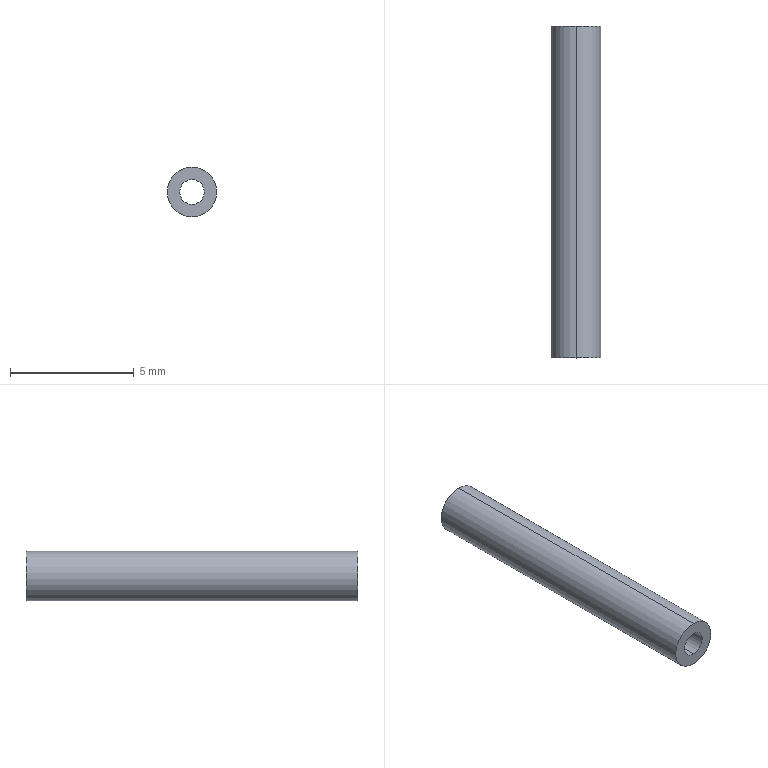Part | SolidWorks | features Extrusion 1 | 1 solid | 6 faces | box 2 x 13.4 x 2 mm | volume 31.573 mm3 | cylinder 4 | plane 2 | commonest cylinder face diameters 1 x2 2 x2
STEP:
#1=CARTESIAN_POINT('',(0.,13.4,-0.5));
#2=VERTEX_POINT('',#1);
#3=CARTESIAN_POINT('',(0.,13.4,0.5));
#4=VERTEX_POINT('',#3);
#5=CARTESIAN_POINT('',(0.,13.4,0.));
#6=DIRECTION('',(0.,1.,0.));
#7=DIRECTION('',(0.,0.,1.));
#8=AXIS2_PLACEMENT_3D('',#5,#6,#7);
#9=CIRCLE('',#8,0.5);
#10=EDGE_CURVE('',#2,#4,#9,.T.);
#11=ORIENTED_EDGE('',*,*,#10,.T.);
#12=CARTESIAN_POINT('',(0.,0.,0.5));
#13=VERTEX_POINT('',#12);
#14=CARTESIAN_POINT('',(0.,13.4,0.5));
#15=DIRECTION('',(0.,-1.,0.));
#16=VECTOR('',#15,1000.);
#17=LINE('',#14,#16);
#18=EDGE_CURVE('',#4,#13,#17,.T.);
#19=ORIENTED_EDGE('',*,*,#18,.T.);
#20=CARTESIAN_POINT('',(0.,0.,-0.5));
#21=VERTEX_POINT('',#20);
#22=CARTESIAN_POINT('',(0.,0.,0.));
#23=DIRECTION('',(0.,1.,0.));
#24=DIRECTION('',(0.,0.,1.));
#25=AXIS2_PLACEMENT_3D('',#22,#23,#24);
#26=CIRCLE('',#25,0.5);
#27=EDGE_CURVE('',#21,#13,#26,.T.);
#28=ORIENTED_EDGE('',*,*,#27,.F.);
#29=CARTESIAN_POINT('',(0.,13.4,-0.5));
#30=DIRECTION('',(0.,-1.,0.));
#31=VECTOR('',#30,1000.);
#32=LINE('',#29,#31);
#33=EDGE_CURVE('',#2,#21,#32,.T.);
#34=ORIENTED_EDGE('',*,*,#33,.F.);
#35=EDGE_LOOP('',(#11,#19,#28,#34));
#36=FACE_OUTER_BOUND('',#35,.T.);
#37=CARTESIAN_POINT('',(0.,13.4,0.));
#38=DIRECTION('',(0.,-1.,0.));
#39=DIRECTION('',(0.,0.,-1.));
#40=AXIS2_PLACEMENT_3D('',#37,#38,#39);
#41=CYLINDRICAL_SURFACE('',#40,0.5);
#42=ADVANCED_FACE('',(#36),#41,.F.);
#43=CARTESIAN_POINT('',(0.,13.4,1.));
#44=VERTEX_POINT('',#43);
#45=CARTESIAN_POINT('',(0.,13.4,-1.));
#46=VERTEX_POINT('',#45);
#47=CARTESIAN_POINT('',(0.,13.4,0.));
#48=DIRECTION('',(0.,1.,0.));
#49=DIRECTION('',(0.,0.,1.));
#50=AXIS2_PLACEMENT_3D('',#47,#48,#49);
#51=CIRCLE('',#50,1.);
#52=EDGE_CURVE('',#44,#46,#51,.T.);
#53=ORIENTED_EDGE('',*,*,#52,.F.);
#54=CARTESIAN_POINT('',(0.,0.,1.));
#55=VERTEX_POINT('',#54);
#56=CARTESIAN_POINT('',(0.,13.4,1.));
#57=DIRECTION('',(0.,-1.,0.));
#58=VECTOR('',#57,1000.);
#59=LINE('',#56,#58);
#60=EDGE_CURVE('',#44,#55,#59,.T.);
#61=ORIENTED_EDGE('',*,*,#60,.T.);
#62=CARTESIAN_POINT('',(0.,0.,-1.));
#63=VERTEX_POINT('',#62);
#64=CARTESIAN_POINT('',(0.,0.,0.));
#65=DIRECTION('',(0.,1.,0.));
#66=DIRECTION('',(0.,0.,1.));
#67=AXIS2_PLACEMENT_3D('',#64,#65,#66);
#68=CIRCLE('',#67,1.);
#69=EDGE_CURVE('',#55,#63,#68,.T.);
#70=ORIENTED_EDGE('',*,*,#69,.T.);
#71=CARTESIAN_POINT('',(0.,13.4,-1.));
#72=DIRECTION('',(0.,-1.,0.));
#73=VECTOR('',#72,1000.);
#74=LINE('',#71,#73);
#75=EDGE_CURVE('',#46,#63,#74,.T.);
#76=ORIENTED_EDGE('',*,*,#75,.F.);
#77=EDGE_LOOP('',(#53,#61,#70,#76));
#78=FACE_OUTER_BOUND('',#77,.T.);
#79=CARTESIAN_POINT('',(0.,13.4,0.));
#80=DIRECTION('',(0.,-1.,0.));
#81=DIRECTION('',(0.,0.,-1.));
#82=AXIS2_PLACEMENT_3D('',#79,#80,#81);
#83=CYLINDRICAL_SURFACE('',#82,1.);
#84=ADVANCED_FACE('',(#78),#83,.T.);
#85=CARTESIAN_POINT('',(0.,13.4,0.));
#86=DIRECTION('',(0.,1.,0.));
#87=DIRECTION('',(0.,0.,1.));
#88=AXIS2_PLACEMENT_3D('',#85,#86,#87);
#89=CIRCLE('',#88,1.);
#90=EDGE_CURVE('',#46,#44,#89,.T.);
#91=ORIENTED_EDGE('',*,*,#90,.T.);
#92=ORIENTED_EDGE('',*,*,#52,.T.);
#93=EDGE_LOOP('',(#91,#92));
#94=FACE_OUTER_BOUND('',#93,.T.);
#95=ORIENTED_EDGE('',*,*,#10,.F.);
#96=CARTESIAN_POINT('',(0.,13.4,0.));
#97=DIRECTION('',(0.,1.,0.));
#98=DIRECTION('',(0.,0.,1.));
#99=AXIS2_PLACEMENT_3D('',#96,#97,#98);
#100=CIRCLE('',#99,0.5);
#101=EDGE_CURVE('',#4,#2,#100,.T.);
#102=ORIENTED_EDGE('',*,*,#101,.F.);
#103=EDGE_LOOP('',(#95,#102));
#104=FACE_BOUND('',#103,.T.);
#105=CARTESIAN_POINT('',(0.,13.4,0.));
#106=DIRECTION('',(0.,1.,0.));
#107=DIRECTION('',(0.,0.,1.));
#108=AXIS2_PLACEMENT_3D('',#105,#106,#107);
#109=PLANE('',#108);
#110=ADVANCED_FACE('',(#94,#104),#109,.T.);
#111=CARTESIAN_POINT('',(0.,0.,0.));
#112=DIRECTION('',(0.,1.,0.));
#113=DIRECTION('',(0.,0.,1.));
#114=AXIS2_PLACEMENT_3D('',#111,#112,#113);
#115=CIRCLE('',#114,1.);
#116=EDGE_CURVE('',#63,#55,#115,.T.);
#117=ORIENTED_EDGE('',*,*,#116,.F.);
#118=ORIENTED_EDGE('',*,*,#69,.F.);
#119=EDGE_LOOP('',(#117,#118));
#120=FACE_OUTER_BOUND('',#119,.T.);
#121=ORIENTED_EDGE('',*,*,#27,.T.);
#122=CARTESIAN_POINT('',(0.,0.,0.));
#123=DIRECTION('',(0.,1.,0.));
#124=DIRECTION('',(0.,0.,1.));
#125=AXIS2_PLACEMENT_3D('',#122,#123,#124);
#126=CIRCLE('',#125,0.5);
#127=EDGE_CURVE('',#13,#21,#126,.T.);
#128=ORIENTED_EDGE('',*,*,#127,.T.);
#129=EDGE_LOOP('',(#121,#128));
#130=FACE_BOUND('',#129,.T.);
#131=CARTESIAN_POINT('',(0.,0.,0.));
#132=DIRECTION('',(0.,1.,0.));
#133=DIRECTION('',(0.,0.,1.));
#134=AXIS2_PLACEMENT_3D('',#131,#132,#133);
#135=PLANE('',#134);
#136=ADVANCED_FACE('',(#120,#130),#135,.F.);
#137=ORIENTED_EDGE('',*,*,#60,.F.);
#138=ORIENTED_EDGE('',*,*,#90,.F.);
#139=ORIENTED_EDGE('',*,*,#75,.T.);
#140=ORIENTED_EDGE('',*,*,#116,.T.);
#141=EDGE_LOOP('',(#137,#138,#139,#140));
#142=FACE_OUTER_BOUND('',#141,.T.);
#143=CARTESIAN_POINT('',(0.,13.4,0.));
#144=DIRECTION('',(0.,-1.,0.));
#145=DIRECTION('',(0.,0.,-1.));
#146=AXIS2_PLACEMENT_3D('',#143,#144,#145);
#147=CYLINDRICAL_SURFACE('',#146,1.);
#148=ADVANCED_FACE('',(#142),#147,.T.);
#149=ORIENTED_EDGE('',*,*,#18,.F.);
#150=ORIENTED_EDGE('',*,*,#101,.T.);
#151=ORIENTED_EDGE('',*,*,#33,.T.);
#152=ORIENTED_EDGE('',*,*,#127,.F.);
#153=EDGE_LOOP('',(#149,#150,#151,#152));
#154=FACE_OUTER_BOUND('',#153,.T.);
#155=CARTESIAN_POINT('',(0.,13.4,0.));
#156=DIRECTION('',(0.,-1.,0.));
#157=DIRECTION('',(0.,0.,-1.));
#158=AXIS2_PLACEMENT_3D('',#155,#156,#157);
#159=CYLINDRICAL_SURFACE('',#158,0.5);
#160=ADVANCED_FACE('',(#154),#159,.F.);
#161=CLOSED_SHELL('',(#42,#84,#110,#136,#148,#160));
#162=MANIFOLD_SOLID_BREP('',#161);
#163=CARTESIAN_POINT('',(0.,0.,0.));
#164=DIRECTION('',(0.,0.,1.));
#165=DIRECTION('',(1.,0.,0.));
#166=AXIS2_PLACEMENT_3D('',#163,#164,#165);
#167=(LENGTH_UNIT()NAMED_UNIT(*)SI_UNIT(.MILLI.,.METRE.));
#168=UNCERTAINTY_MEASURE_WITH_UNIT(LENGTH_MEASURE(0.00001),#167,'','');
#169=(NAMED_UNIT(*)PLANE_ANGLE_UNIT()SI_UNIT($,.RADIAN.));
#170=(NAMED_UNIT(*)SI_UNIT($,.STERADIAN.)SOLID_ANGLE_UNIT());
#171=(GEOMETRIC_REPRESENTATION_CONTEXT(3)GLOBAL_UNCERTAINTY_ASSIGNED_CONTEXT((#168))GLOBAL_UNIT_ASSIGNED_CONTEXT((#167,#169,#170))REPRESENTATION_CONTEXT('',''));
#172=ADVANCED_BREP_SHAPE_REPRESENTATION('',(#162,#166),#171);